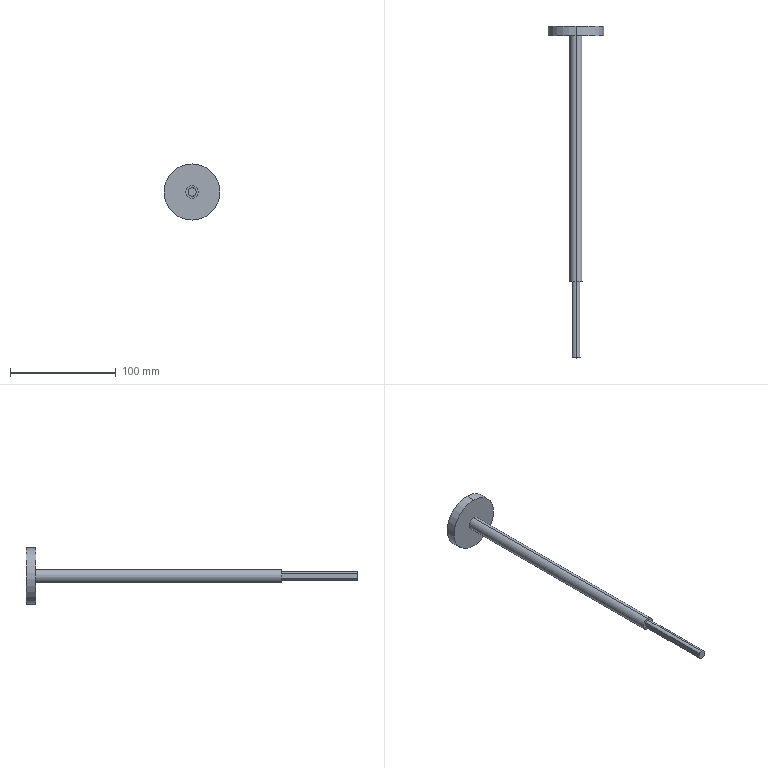Part | STEP file | 1 solid | 12 faces | box 53 x 313.9 x 53 mm | volume 49554 mm3 | cylinder 7 | plane 5 | commonest cylinder face diameters 8 x3 12 x2 53 x2
STEP:
#1=CARTESIAN_POINT('',(0.,0.,0.));
#2=DIRECTION('',(0.,0.,1.));
#3=DIRECTION('',(1.,0.,0.));
#4=AXIS2_PLACEMENT_3D('',#1,#2,#3);
#5=CARTESIAN_POINT('',(0.,313.9,-26.5));
#6=VERTEX_POINT('',#5);
#7=CARTESIAN_POINT('',(0.,313.9,26.5));
#8=VERTEX_POINT('',#7);
#9=CARTESIAN_POINT('',(0.,313.9,0.));
#10=DIRECTION('',(0.,-1.,0.));
#11=DIRECTION('',(0.,0.,-1.));
#12=AXIS2_PLACEMENT_3D('',#9,#10,#11);
#13=CIRCLE('',#12,26.5);
#14=CARTESIAN_POINT('',(0.,0.,0.));
#15=DIRECTION('',(0.,-1.,0.));
#16=DIRECTION('',(0.,0.,-1.));
#17=AXIS2_PLACEMENT_3D('',#14,#15,#16);
#18=CYLINDRICAL_SURFACE('',#17,26.5);
#19=CARTESIAN_POINT('',(0.,-313.9));
#20=DIRECTION('',(1.,0.));
#21=VECTOR('',#20,1.);
#22=LINE('',#19,#21);
#23=(GEOMETRIC_REPRESENTATION_CONTEXT(2)PARAMETRIC_REPRESENTATION_CONTEXT()REPRESENTATION_CONTEXT('',''));
#24=DEFINITIONAL_REPRESENTATION('',(#22),#23);
#25=PCURVE('',#18,#24);
#26=CARTESIAN_POINT('',(26.5,313.9,0.));
#27=DIRECTION('',(0.,1.,0.));
#28=DIRECTION('',(0.,0.,1.));
#29=AXIS2_PLACEMENT_3D('',#26,#27,#28);
#30=PLANE('',#29);
#31=CARTESIAN_POINT('',(-26.5,-26.5));
#32=CARTESIAN_POINT('',(-26.5,19.399));
#33=CARTESIAN_POINT('',(13.25,-3.55));
#34=CARTESIAN_POINT('',(53.,-26.5));
#35=CARTESIAN_POINT('',(13.25,-49.45));
#36=CARTESIAN_POINT('',(-26.5,-72.399));
#37=CARTESIAN_POINT('',(-26.5,-26.5));
#38=(BOUNDED_CURVE()B_SPLINE_CURVE(2,(#31,#32,#33,#34,#35,#36,#37),.UNSPECIFIED.,.T.,.F.)B_SPLINE_CURVE_WITH_KNOTS((1,2,2,2,2,1),(-2.094,0.,2.094,4.189,6.283,8.378),.UNSPECIFIED.)CURVE()GEOMETRIC_REPRESENTATION_ITEM()RATIONAL_B_SPLINE_CURVE((1.,0.5,1.,0.5,1.,0.5,1.))REPRESENTATION_ITEM(''));
#39=(GEOMETRIC_REPRESENTATION_CONTEXT(2)PARAMETRIC_REPRESENTATION_CONTEXT()REPRESENTATION_CONTEXT('',''));
#40=DEFINITIONAL_REPRESENTATION('',(#38),#39);
#41=PCURVE('',#30,#40);
#42=SURFACE_CURVE('',#13,(#25,#41),.PCURVE_S1.);
#43=EDGE_CURVE('',#6,#8,#42,.T.);
#44=ORIENTED_EDGE('',*,*,#43,.T.);
#45=CARTESIAN_POINT('',(0.,304.9,26.5));
#46=VERTEX_POINT('',#45);
#47=CARTESIAN_POINT('',(0.,0.,26.5));
#48=DIRECTION('',(0.,-1.,0.));
#49=VECTOR('',#48,1.);
#50=LINE('',#47,#49);
#51=CARTESIAN_POINT('',(3.142,0.));
#52=DIRECTION('',(0.,1.));
#53=VECTOR('',#52,1.);
#54=LINE('',#51,#53);
#55=(GEOMETRIC_REPRESENTATION_CONTEXT(2)PARAMETRIC_REPRESENTATION_CONTEXT()REPRESENTATION_CONTEXT('',''));
#56=DEFINITIONAL_REPRESENTATION('',(#54),#55);
#57=PCURVE('',#18,#56);
#58=CARTESIAN_POINT('',(0.,0.,0.));
#59=DIRECTION('',(0.,-1.,0.));
#60=DIRECTION('',(0.,0.,-1.));
#61=AXIS2_PLACEMENT_3D('',#58,#59,#60);
#62=CYLINDRICAL_SURFACE('',#61,26.5);
#63=CARTESIAN_POINT('',(3.142,0.));
#64=DIRECTION('',(0.,1.));
#65=VECTOR('',#64,1.);
#66=LINE('',#63,#65);
#67=(GEOMETRIC_REPRESENTATION_CONTEXT(2)PARAMETRIC_REPRESENTATION_CONTEXT()REPRESENTATION_CONTEXT('',''));
#68=DEFINITIONAL_REPRESENTATION('',(#66),#67);
#69=PCURVE('',#62,#68);
#70=SURFACE_CURVE('',#50,(#57,#69),.PCURVE_S1.);
#71=EDGE_CURVE('',#8,#46,#70,.T.);
#72=ORIENTED_EDGE('',*,*,#71,.T.);
#73=CARTESIAN_POINT('',(0.,304.9,-26.5));
#74=VERTEX_POINT('',#73);
#75=CARTESIAN_POINT('',(0.,304.9,0.));
#76=DIRECTION('',(0.,-1.,0.));
#77=DIRECTION('',(0.,0.,-1.));
#78=AXIS2_PLACEMENT_3D('',#75,#76,#77);
#79=CIRCLE('',#78,26.5);
#80=CARTESIAN_POINT('',(0.,-304.9));
#81=DIRECTION('',(1.,0.));
#82=VECTOR('',#81,1.);
#83=LINE('',#80,#82);
#84=(GEOMETRIC_REPRESENTATION_CONTEXT(2)PARAMETRIC_REPRESENTATION_CONTEXT()REPRESENTATION_CONTEXT('',''));
#85=DEFINITIONAL_REPRESENTATION('',(#83),#84);
#86=PCURVE('',#18,#85);
#87=CARTESIAN_POINT('',(6.,304.9,0.));
#88=DIRECTION('',(0.,-1.,0.));
#89=DIRECTION('',(0.,0.,-1.));
#90=AXIS2_PLACEMENT_3D('',#87,#88,#89);
#91=PLANE('',#90);
#92=CARTESIAN_POINT('',(0.,-6.));
#93=DIRECTION('',(1.,0.));
#94=AXIS2_PLACEMENT_2D('',#92,#93);
#95=CIRCLE('',#94,26.5);
#96=(GEOMETRIC_REPRESENTATION_CONTEXT(2)PARAMETRIC_REPRESENTATION_CONTEXT()REPRESENTATION_CONTEXT('',''));
#97=DEFINITIONAL_REPRESENTATION('',(#95),#96);
#98=PCURVE('',#91,#97);
#99=SURFACE_CURVE('',#79,(#86,#98),.PCURVE_S1.);
#100=EDGE_CURVE('',#74,#46,#99,.T.);
#101=ORIENTED_EDGE('',*,*,#100,.F.);
#102=CARTESIAN_POINT('',(0.,0.,-26.5));
#103=DIRECTION('',(0.,-1.,0.));
#104=VECTOR('',#103,1.);
#105=LINE('',#102,#104);
#106=CARTESIAN_POINT('',(0.,0.));
#107=DIRECTION('',(0.,1.));
#108=VECTOR('',#107,1.);
#109=LINE('',#106,#108);
#110=(GEOMETRIC_REPRESENTATION_CONTEXT(2)PARAMETRIC_REPRESENTATION_CONTEXT()REPRESENTATION_CONTEXT('',''));
#111=DEFINITIONAL_REPRESENTATION('',(#109),#110);
#112=PCURVE('',#18,#111);
#113=CARTESIAN_POINT('',(6.283,0.));
#114=DIRECTION('',(0.,1.));
#115=VECTOR('',#114,1.);
#116=LINE('',#113,#115);
#117=(GEOMETRIC_REPRESENTATION_CONTEXT(2)PARAMETRIC_REPRESENTATION_CONTEXT()REPRESENTATION_CONTEXT('',''));
#118=DEFINITIONAL_REPRESENTATION('',(#116),#117);
#119=PCURVE('',#62,#118);
#120=SURFACE_CURVE('',#105,(#112,#119),.PCURVE_S1.);
#121=EDGE_CURVE('',#6,#74,#120,.T.);
#122=ORIENTED_EDGE('',*,*,#121,.F.);
#123=EDGE_LOOP('',(#44,#72,#101,#122));
#124=FACE_BOUND('',#123,.T.);
#125=ADVANCED_FACE('',(#124),#18,.T.);
#126=CARTESIAN_POINT('',(0.,304.9,-6.));
#127=VERTEX_POINT('',#126);
#128=CARTESIAN_POINT('',(0.,304.9,6.));
#129=VERTEX_POINT('',#128);
#130=CARTESIAN_POINT('',(0.,304.9,0.));
#131=DIRECTION('',(0.,-1.,0.));
#132=DIRECTION('',(0.,0.,-1.));
#133=AXIS2_PLACEMENT_3D('',#130,#131,#132);
#134=CIRCLE('',#133,6.);
#135=CARTESIAN_POINT('',(0.,0.,0.));
#136=DIRECTION('',(0.,-1.,0.));
#137=DIRECTION('',(0.,0.,-1.));
#138=AXIS2_PLACEMENT_3D('',#135,#136,#137);
#139=CYLINDRICAL_SURFACE('',#138,6.);
#140=CARTESIAN_POINT('',(0.,-304.9));
#141=DIRECTION('',(1.,0.));
#142=VECTOR('',#141,1.);
#143=LINE('',#140,#142);
#144=(GEOMETRIC_REPRESENTATION_CONTEXT(2)PARAMETRIC_REPRESENTATION_CONTEXT()REPRESENTATION_CONTEXT('',''));
#145=DEFINITIONAL_REPRESENTATION('',(#143),#144);
#146=PCURVE('',#139,#145);
#147=CARTESIAN_POINT('',(0.,-6.));
#148=DIRECTION('',(1.,0.));
#149=AXIS2_PLACEMENT_2D('',#147,#148);
#150=CIRCLE('',#149,6.);
#151=(GEOMETRIC_REPRESENTATION_CONTEXT(2)PARAMETRIC_REPRESENTATION_CONTEXT()REPRESENTATION_CONTEXT('',''));
#152=DEFINITIONAL_REPRESENTATION('',(#150),#151);
#153=PCURVE('',#91,#152);
#154=SURFACE_CURVE('',#134,(#146,#153),.PCURVE_S1.);
#155=EDGE_CURVE('',#127,#129,#154,.T.);
#156=ORIENTED_EDGE('',*,*,#155,.T.);
#157=CARTESIAN_POINT('',(0.,72.,6.));
#158=VERTEX_POINT('',#157);
#159=CARTESIAN_POINT('',(0.,0.,6.));
#160=DIRECTION('',(0.,-1.,0.));
#161=VECTOR('',#160,1.);
#162=LINE('',#159,#161);
#163=CARTESIAN_POINT('',(3.142,0.));
#164=DIRECTION('',(0.,1.));
#165=VECTOR('',#164,1.);
#166=LINE('',#163,#165);
#167=(GEOMETRIC_REPRESENTATION_CONTEXT(2)PARAMETRIC_REPRESENTATION_CONTEXT()REPRESENTATION_CONTEXT('',''));
#168=DEFINITIONAL_REPRESENTATION('',(#166),#167);
#169=PCURVE('',#139,#168);
#170=CARTESIAN_POINT('',(0.,0.,0.));
#171=DIRECTION('',(0.,-1.,0.));
#172=DIRECTION('',(0.,0.,-1.));
#173=AXIS2_PLACEMENT_3D('',#170,#171,#172);
#174=CYLINDRICAL_SURFACE('',#173,6.);
#175=CARTESIAN_POINT('',(3.142,0.));
#176=DIRECTION('',(0.,1.));
#177=VECTOR('',#176,1.);
#178=LINE('',#175,#177);
#179=(GEOMETRIC_REPRESENTATION_CONTEXT(2)PARAMETRIC_REPRESENTATION_CONTEXT()REPRESENTATION_CONTEXT('',''));
#180=DEFINITIONAL_REPRESENTATION('',(#178),#179);
#181=PCURVE('',#174,#180);
#182=SURFACE_CURVE('',#162,(#169,#181),.PCURVE_S1.);
#183=EDGE_CURVE('',#129,#158,#182,.T.);
#184=ORIENTED_EDGE('',*,*,#183,.T.);
#185=CARTESIAN_POINT('',(0.,72.,-6.));
#186=VERTEX_POINT('',#185);
#187=CARTESIAN_POINT('',(0.,72.,0.));
#188=DIRECTION('',(0.,-1.,0.));
#189=DIRECTION('',(0.,0.,-1.));
#190=AXIS2_PLACEMENT_3D('',#187,#188,#189);
#191=CIRCLE('',#190,6.);
#192=CARTESIAN_POINT('',(0.,-72.));
#193=DIRECTION('',(1.,0.));
#194=VECTOR('',#193,1.);
#195=LINE('',#192,#194);
#196=(GEOMETRIC_REPRESENTATION_CONTEXT(2)PARAMETRIC_REPRESENTATION_CONTEXT()REPRESENTATION_CONTEXT('',''));
#197=DEFINITIONAL_REPRESENTATION('',(#195),#196);
#198=PCURVE('',#139,#197);
#199=CARTESIAN_POINT('',(4.,72.,0.));
#200=DIRECTION('',(0.,-1.,0.));
#201=DIRECTION('',(0.,0.,-1.));
#202=AXIS2_PLACEMENT_3D('',#199,#200,#201);
#203=PLANE('',#202);
#204=CARTESIAN_POINT('',(0.,-4.));
#205=DIRECTION('',(1.,0.));
#206=AXIS2_PLACEMENT_2D('',#204,#205);
#207=CIRCLE('',#206,6.);
#208=(GEOMETRIC_REPRESENTATION_CONTEXT(2)PARAMETRIC_REPRESENTATION_CONTEXT()REPRESENTATION_CONTEXT('',''));
#209=DEFINITIONAL_REPRESENTATION('',(#207),#208);
#210=PCURVE('',#203,#209);
#211=SURFACE_CURVE('',#191,(#198,#210),.PCURVE_S1.);
#212=EDGE_CURVE('',#186,#158,#211,.T.);
#213=ORIENTED_EDGE('',*,*,#212,.F.);
#214=CARTESIAN_POINT('',(0.,0.,-6.));
#215=DIRECTION('',(0.,-1.,0.));
#216=VECTOR('',#215,1.);
#217=LINE('',#214,#216);
#218=CARTESIAN_POINT('',(0.,0.));
#219=DIRECTION('',(0.,1.));
#220=VECTOR('',#219,1.);
#221=LINE('',#218,#220);
#222=(GEOMETRIC_REPRESENTATION_CONTEXT(2)PARAMETRIC_REPRESENTATION_CONTEXT()REPRESENTATION_CONTEXT('',''));
#223=DEFINITIONAL_REPRESENTATION('',(#221),#222);
#224=PCURVE('',#139,#223);
#225=CARTESIAN_POINT('',(6.283,0.));
#226=DIRECTION('',(0.,1.));
#227=VECTOR('',#226,1.);
#228=LINE('',#225,#227);
#229=(GEOMETRIC_REPRESENTATION_CONTEXT(2)PARAMETRIC_REPRESENTATION_CONTEXT()REPRESENTATION_CONTEXT('',''));
#230=DEFINITIONAL_REPRESENTATION('',(#228),#229);
#231=PCURVE('',#174,#230);
#232=SURFACE_CURVE('',#217,(#224,#231),.PCURVE_S1.);
#233=EDGE_CURVE('',#127,#186,#232,.T.);
#234=ORIENTED_EDGE('',*,*,#233,.F.);
#235=EDGE_LOOP('',(#156,#184,#213,#234));
#236=FACE_BOUND('',#235,.T.);
#237=ADVANCED_FACE('',(#236),#139,.T.);
#238=CARTESIAN_POINT('',(0.,72.,-4.));
#239=VERTEX_POINT('',#238);
#240=CARTESIAN_POINT('',(0.,72.,4.));
#241=VERTEX_POINT('',#240);
#242=CARTESIAN_POINT('',(0.,72.,0.));
#243=DIRECTION('',(0.,-1.,0.));
#244=DIRECTION('',(0.,0.,-1.));
#245=AXIS2_PLACEMENT_3D('',#242,#243,#244);
#246=CIRCLE('',#245,4.);
#247=CARTESIAN_POINT('',(0.,0.,0.));
#248=DIRECTION('',(0.,-1.,0.));
#249=DIRECTION('',(0.,0.,-1.));
#250=AXIS2_PLACEMENT_3D('',#247,#248,#249);
#251=CYLINDRICAL_SURFACE('',#250,4.);
#252=CARTESIAN_POINT('',(0.,-72.));
#253=DIRECTION('',(1.,0.));
#254=VECTOR('',#253,1.);
#255=LINE('',#252,#254);
#256=(GEOMETRIC_REPRESENTATION_CONTEXT(2)PARAMETRIC_REPRESENTATION_CONTEXT()REPRESENTATION_CONTEXT('',''));
#257=DEFINITIONAL_REPRESENTATION('',(#255),#256);
#258=PCURVE('',#251,#257);
#259=CARTESIAN_POINT('',(0.,-4.));
#260=DIRECTION('',(1.,0.));
#261=AXIS2_PLACEMENT_2D('',#259,#260);
#262=CIRCLE('',#261,4.);
#263=(GEOMETRIC_REPRESENTATION_CONTEXT(2)PARAMETRIC_REPRESENTATION_CONTEXT()REPRESENTATION_CONTEXT('',''));
#264=DEFINITIONAL_REPRESENTATION('',(#262),#263);
#265=PCURVE('',#203,#264);
#266=SURFACE_CURVE('',#246,(#258,#265),.PCURVE_S1.);
#267=EDGE_CURVE('',#239,#241,#266,.T.);
#268=ORIENTED_EDGE('',*,*,#267,.T.);
#269=CARTESIAN_POINT('',(0.,0.,4.));
#270=VERTEX_POINT('',#269);
#271=CARTESIAN_POINT('',(0.,0.,4.));
#272=DIRECTION('',(0.,-1.,0.));
#273=VECTOR('',#272,1.);
#274=LINE('',#271,#273);
#275=CARTESIAN_POINT('',(3.142,0.));
#276=DIRECTION('',(0.,1.));
#277=VECTOR('',#276,1.);
#278=LINE('',#275,#277);
#279=(GEOMETRIC_REPRESENTATION_CONTEXT(2)PARAMETRIC_REPRESENTATION_CONTEXT()REPRESENTATION_CONTEXT('',''));
#280=DEFINITIONAL_REPRESENTATION('',(#278),#279);
#281=PCURVE('',#251,#280);
#282=CARTESIAN_POINT('',(0.,0.,0.));
#283=DIRECTION('',(0.,-1.,0.));
#284=DIRECTION('',(0.,0.,-1.));
#285=AXIS2_PLACEMENT_3D('',#282,#283,#284);
#286=CYLINDRICAL_SURFACE('',#285,4.);
#287=CARTESIAN_POINT('',(3.142,0.));
#288=DIRECTION('',(0.,1.));
#289=VECTOR('',#288,1.);
#290=LINE('',#287,#289);
#291=(GEOMETRIC_REPRESENTATION_CONTEXT(2)PARAMETRIC_REPRESENTATION_CONTEXT()REPRESENTATION_CONTEXT('',''));
#292=DEFINITIONAL_REPRESENTATION('',(#290),#291);
#293=PCURVE('',#286,#292);
#294=SURFACE_CURVE('',#274,(#281,#293),.PCURVE_S1.);
#295=EDGE_CURVE('',#241,#270,#294,.T.);
#296=ORIENTED_EDGE('',*,*,#295,.T.);
#297=CARTESIAN_POINT('',(0.,0.,-4.));
#298=VERTEX_POINT('',#297);
#299=CARTESIAN_POINT('',(0.,0.,0.));
#300=DIRECTION('',(0.,-1.,0.));
#301=DIRECTION('',(0.,0.,-1.));
#302=AXIS2_PLACEMENT_3D('',#299,#300,#301);
#303=CIRCLE('',#302,4.);
#304=CARTESIAN_POINT('',(0.,0.));
#305=DIRECTION('',(1.,0.));
#306=VECTOR('',#305,1.);
#307=LINE('',#304,#306);
#308=(GEOMETRIC_REPRESENTATION_CONTEXT(2)PARAMETRIC_REPRESENTATION_CONTEXT()REPRESENTATION_CONTEXT('',''));
#309=DEFINITIONAL_REPRESENTATION('',(#307),#308);
#310=PCURVE('',#251,#309);
#311=CARTESIAN_POINT('',(0.,0.,0.));
#312=DIRECTION('',(0.,-1.,0.));
#313=DIRECTION('',(0.,0.,-1.));
#314=AXIS2_PLACEMENT_3D('',#311,#312,#313);
#315=PLANE('',#314);
#316=CARTESIAN_POINT('',(0.,0.));
#317=DIRECTION('',(1.,0.));
#318=AXIS2_PLACEMENT_2D('',#316,#317);
#319=CIRCLE('',#318,4.);
#320=(GEOMETRIC_REPRESENTATION_CONTEXT(2)PARAMETRIC_REPRESENTATION_CONTEXT()REPRESENTATION_CONTEXT('',''));
#321=DEFINITIONAL_REPRESENTATION('',(#319),#320);
#322=PCURVE('',#315,#321);
#323=SURFACE_CURVE('',#303,(#310,#322),.PCURVE_S1.);
#324=EDGE_CURVE('',#298,#270,#323,.T.);
#325=ORIENTED_EDGE('',*,*,#324,.F.);
#326=CARTESIAN_POINT('',(0.,0.,-4.));
#327=DIRECTION('',(0.,-1.,0.));
#328=VECTOR('',#327,1.);
#329=LINE('',#326,#328);
#330=CARTESIAN_POINT('',(0.,0.));
#331=DIRECTION('',(0.,1.));
#332=VECTOR('',#331,1.);
#333=LINE('',#330,#332);
#334=(GEOMETRIC_REPRESENTATION_CONTEXT(2)PARAMETRIC_REPRESENTATION_CONTEXT()REPRESENTATION_CONTEXT('',''));
#335=DEFINITIONAL_REPRESENTATION('',(#333),#334);
#336=PCURVE('',#251,#335);
#337=CARTESIAN_POINT('',(0.,0.,0.));
#338=DIRECTION('',(0.,-1.,0.));
#339=DIRECTION('',(0.,0.,-1.));
#340=AXIS2_PLACEMENT_3D('',#337,#338,#339);
#341=CYLINDRICAL_SURFACE('',#340,4.);
#342=CARTESIAN_POINT('',(6.283,0.));
#343=DIRECTION('',(0.,1.));
#344=VECTOR('',#343,1.);
#345=LINE('',#342,#344);
#346=(GEOMETRIC_REPRESENTATION_CONTEXT(2)PARAMETRIC_REPRESENTATION_CONTEXT()REPRESENTATION_CONTEXT('',''));
#347=DEFINITIONAL_REPRESENTATION('',(#345),#346);
#348=PCURVE('',#341,#347);
#349=SURFACE_CURVE('',#329,(#336,#348),.PCURVE_S1.);
#350=EDGE_CURVE('',#239,#298,#349,.T.);
#351=ORIENTED_EDGE('',*,*,#350,.F.);
#352=EDGE_LOOP('',(#268,#296,#325,#351));
#353=FACE_BOUND('',#352,.T.);
#354=ADVANCED_FACE('',(#353),#251,.T.);
#355=CARTESIAN_POINT('',(-3.,72.,-2.646));
#356=VERTEX_POINT('',#355);
#357=CARTESIAN_POINT('',(0.,72.,0.));
#358=DIRECTION('',(0.,-1.,0.));
#359=DIRECTION('',(0.,0.,-1.));
#360=AXIS2_PLACEMENT_3D('',#357,#358,#359);
#361=CIRCLE('',#360,4.);
#362=CARTESIAN_POINT('',(0.,-72.));
#363=DIRECTION('',(1.,0.));
#364=VECTOR('',#363,1.);
#365=LINE('',#362,#364);
#366=(GEOMETRIC_REPRESENTATION_CONTEXT(2)PARAMETRIC_REPRESENTATION_CONTEXT()REPRESENTATION_CONTEXT('',''));
#367=DEFINITIONAL_REPRESENTATION('',(#365),#366);
#368=PCURVE('',#341,#367);
#369=CARTESIAN_POINT('',(0.,-4.));
#370=DIRECTION('',(1.,0.));
#371=AXIS2_PLACEMENT_2D('',#369,#370);
#372=CIRCLE('',#371,4.);
#373=(GEOMETRIC_REPRESENTATION_CONTEXT(2)PARAMETRIC_REPRESENTATION_CONTEXT()REPRESENTATION_CONTEXT('',''));
#374=DEFINITIONAL_REPRESENTATION('',(#372),#373);
#375=PCURVE('',#203,#374);
#376=SURFACE_CURVE('',#361,(#368,#375),.PCURVE_S1.);
#377=EDGE_CURVE('',#356,#239,#376,.T.);
#378=ORIENTED_EDGE('',*,*,#377,.T.);
#379=ORIENTED_EDGE('',*,*,#350,.T.);
#380=CARTESIAN_POINT('',(-3.,0.,-2.646));
#381=VERTEX_POINT('',#380);
#382=CARTESIAN_POINT('',(0.,0.,0.));
#383=DIRECTION('',(0.,-1.,0.));
#384=DIRECTION('',(0.,0.,-1.));
#385=AXIS2_PLACEMENT_3D('',#382,#383,#384);
#386=CIRCLE('',#385,4.);
#387=CARTESIAN_POINT('',(0.,0.));
#388=DIRECTION('',(1.,0.));
#389=VECTOR('',#388,1.);
#390=LINE('',#387,#389);
#391=(GEOMETRIC_REPRESENTATION_CONTEXT(2)PARAMETRIC_REPRESENTATION_CONTEXT()REPRESENTATION_CONTEXT('',''));
#392=DEFINITIONAL_REPRESENTATION('',(#390),#391);
#393=PCURVE('',#341,#392);
#394=CARTESIAN_POINT('',(0.,0.));
#395=DIRECTION('',(1.,0.));
#396=AXIS2_PLACEMENT_2D('',#394,#395);
#397=CIRCLE('',#396,4.);
#398=(GEOMETRIC_REPRESENTATION_CONTEXT(2)PARAMETRIC_REPRESENTATION_CONTEXT()REPRESENTATION_CONTEXT('',''));
#399=DEFINITIONAL_REPRESENTATION('',(#397),#398);
#400=PCURVE('',#315,#399);
#401=SURFACE_CURVE('',#386,(#393,#400),.PCURVE_S1.);
#402=EDGE_CURVE('',#381,#298,#401,.T.);
#403=ORIENTED_EDGE('',*,*,#402,.F.);
#404=CARTESIAN_POINT('',(-3.,0.,-2.646));
#405=DIRECTION('',(0.,-1.,0.));
#406=VECTOR('',#405,1.);
#407=LINE('',#404,#406);
#408=CARTESIAN_POINT('',(5.435,0.));
#409=DIRECTION('',(0.,1.));
#410=VECTOR('',#409,1.);
#411=LINE('',#408,#410);
#412=(GEOMETRIC_REPRESENTATION_CONTEXT(2)PARAMETRIC_REPRESENTATION_CONTEXT()REPRESENTATION_CONTEXT('',''));
#413=DEFINITIONAL_REPRESENTATION('',(#411),#412);
#414=PCURVE('',#341,#413);
#415=CARTESIAN_POINT('',(-3.,95.111,11.649));
#416=DIRECTION('',(1.,0.,0.));
#417=DIRECTION('',(0.,0.,-1.));
#418=AXIS2_PLACEMENT_3D('',#415,#416,#417);
#419=PLANE('',#418);
#420=CARTESIAN_POINT('',(14.294,-95.111));
#421=DIRECTION('',(0.,-1.));
#422=VECTOR('',#421,1.);
#423=LINE('',#420,#422);
#424=(GEOMETRIC_REPRESENTATION_CONTEXT(2)PARAMETRIC_REPRESENTATION_CONTEXT()REPRESENTATION_CONTEXT('',''));
#425=DEFINITIONAL_REPRESENTATION('',(#423),#424);
#426=PCURVE('',#419,#425);
#427=SURFACE_CURVE('',#407,(#414,#426),.PCURVE_S1.);
#428=EDGE_CURVE('',#356,#381,#427,.T.);
#429=ORIENTED_EDGE('',*,*,#428,.F.);
#430=EDGE_LOOP('',(#378,#379,#403,#429));
#431=FACE_BOUND('',#430,.T.);
#432=ADVANCED_FACE('',(#431),#341,.T.);
#433=CARTESIAN_POINT('',(-3.,0.,2.646));
#434=VERTEX_POINT('',#433);
#435=CARTESIAN_POINT('',(-3.,0.,11.649));
#436=DIRECTION('',(0.,0.,1.));
#437=VECTOR('',#436,1.);
#438=LINE('',#435,#437);
#439=CARTESIAN_POINT('',(-11.649,-3.));
#440=DIRECTION('',(-1.,0.));
#441=VECTOR('',#440,1.);
#442=LINE('',#439,#441);
#443=(GEOMETRIC_REPRESENTATION_CONTEXT(2)PARAMETRIC_REPRESENTATION_CONTEXT()REPRESENTATION_CONTEXT('',''));
#444=DEFINITIONAL_REPRESENTATION('',(#442),#443);
#445=PCURVE('',#315,#444);
#446=CARTESIAN_POINT('',(0.,-95.111));
#447=DIRECTION('',(-1.,0.));
#448=VECTOR('',#447,1.);
#449=LINE('',#446,#448);
#450=(GEOMETRIC_REPRESENTATION_CONTEXT(2)PARAMETRIC_REPRESENTATION_CONTEXT()REPRESENTATION_CONTEXT('',''));
#451=DEFINITIONAL_REPRESENTATION('',(#449),#450);
#452=PCURVE('',#419,#451);
#453=SURFACE_CURVE('',#438,(#445,#452),.PCURVE_S1.);
#454=EDGE_CURVE('',#381,#434,#453,.T.);
#455=ORIENTED_EDGE('',*,*,#454,.F.);
#456=ORIENTED_EDGE('',*,*,#402,.T.);
#457=ORIENTED_EDGE('',*,*,#324,.T.);
#458=CARTESIAN_POINT('',(0.,0.,0.));
#459=DIRECTION('',(0.,-1.,0.));
#460=DIRECTION('',(0.,0.,-1.));
#461=AXIS2_PLACEMENT_3D('',#458,#459,#460);
#462=CIRCLE('',#461,4.);
#463=CARTESIAN_POINT('',(0.,0.));
#464=DIRECTION('',(1.,0.));
#465=AXIS2_PLACEMENT_2D('',#463,#464);
#466=CIRCLE('',#465,4.);
#467=(GEOMETRIC_REPRESENTATION_CONTEXT(2)PARAMETRIC_REPRESENTATION_CONTEXT()REPRESENTATION_CONTEXT('',''));
#468=DEFINITIONAL_REPRESENTATION('',(#466),#467);
#469=PCURVE('',#315,#468);
#470=CARTESIAN_POINT('',(0.,0.));
#471=DIRECTION('',(1.,0.));
#472=VECTOR('',#471,1.);
#473=LINE('',#470,#472);
#474=(GEOMETRIC_REPRESENTATION_CONTEXT(2)PARAMETRIC_REPRESENTATION_CONTEXT()REPRESENTATION_CONTEXT('',''));
#475=DEFINITIONAL_REPRESENTATION('',(#473),#474);
#476=PCURVE('',#286,#475);
#477=SURFACE_CURVE('',#462,(#469,#476),.PCURVE_S1.);
#478=EDGE_CURVE('',#270,#434,#477,.T.);
#479=ORIENTED_EDGE('',*,*,#478,.T.);
#480=EDGE_LOOP('',(#455,#456,#457,#479));
#481=FACE_BOUND('',#480,.T.);
#482=ADVANCED_FACE('',(#481),#315,.T.);
#483=ORIENTED_EDGE('',*,*,#295,.F.);
#484=CARTESIAN_POINT('',(-3.,72.,2.646));
#485=VERTEX_POINT('',#484);
#486=CARTESIAN_POINT('',(0.,72.,0.));
#487=DIRECTION('',(0.,-1.,0.));
#488=DIRECTION('',(0.,0.,-1.));
#489=AXIS2_PLACEMENT_3D('',#486,#487,#488);
#490=CIRCLE('',#489,4.);
#491=CARTESIAN_POINT('',(0.,-72.));
#492=DIRECTION('',(1.,0.));
#493=VECTOR('',#492,1.);
#494=LINE('',#491,#493);
#495=(GEOMETRIC_REPRESENTATION_CONTEXT(2)PARAMETRIC_REPRESENTATION_CONTEXT()REPRESENTATION_CONTEXT('',''));
#496=DEFINITIONAL_REPRESENTATION('',(#494),#495);
#497=PCURVE('',#286,#496);
#498=CARTESIAN_POINT('',(0.,-4.));
#499=DIRECTION('',(1.,0.));
#500=AXIS2_PLACEMENT_2D('',#498,#499);
#501=CIRCLE('',#500,4.);
#502=(GEOMETRIC_REPRESENTATION_CONTEXT(2)PARAMETRIC_REPRESENTATION_CONTEXT()REPRESENTATION_CONTEXT('',''));
#503=DEFINITIONAL_REPRESENTATION('',(#501),#502);
#504=PCURVE('',#203,#503);
#505=SURFACE_CURVE('',#490,(#497,#504),.PCURVE_S1.);
#506=EDGE_CURVE('',#241,#485,#505,.T.);
#507=ORIENTED_EDGE('',*,*,#506,.T.);
#508=CARTESIAN_POINT('',(-3.,0.,2.646));
#509=DIRECTION('',(0.,1.,0.));
#510=VECTOR('',#509,1.);
#511=LINE('',#508,#510);
#512=CARTESIAN_POINT('',(3.99,0.));
#513=DIRECTION('',(0.,-1.));
#514=VECTOR('',#513,1.);
#515=LINE('',#512,#514);
#516=(GEOMETRIC_REPRESENTATION_CONTEXT(2)PARAMETRIC_REPRESENTATION_CONTEXT()REPRESENTATION_CONTEXT('',''));
#517=DEFINITIONAL_REPRESENTATION('',(#515),#516);
#518=PCURVE('',#286,#517);
#519=CARTESIAN_POINT('',(9.003,-95.111));
#520=DIRECTION('',(0.,1.));
#521=VECTOR('',#520,1.);
#522=LINE('',#519,#521);
#523=(GEOMETRIC_REPRESENTATION_CONTEXT(2)PARAMETRIC_REPRESENTATION_CONTEXT()REPRESENTATION_CONTEXT('',''));
#524=DEFINITIONAL_REPRESENTATION('',(#522),#523);
#525=PCURVE('',#419,#524);
#526=SURFACE_CURVE('',#511,(#518,#525),.PCURVE_S1.);
#527=EDGE_CURVE('',#434,#485,#526,.T.);
#528=ORIENTED_EDGE('',*,*,#527,.F.);
#529=ORIENTED_EDGE('',*,*,#478,.F.);
#530=EDGE_LOOP('',(#483,#507,#528,#529));
#531=FACE_BOUND('',#530,.T.);
#532=ADVANCED_FACE('',(#531),#286,.T.);
#533=ORIENTED_EDGE('',*,*,#377,.F.);
#534=CARTESIAN_POINT('',(-3.,72.,11.649));
#535=DIRECTION('',(0.,0.,-1.));
#536=VECTOR('',#535,1.);
#537=LINE('',#534,#536);
#538=CARTESIAN_POINT('',(-11.649,-7.));
#539=DIRECTION('',(1.,0.));
#540=VECTOR('',#539,1.);
#541=LINE('',#538,#540);
#542=(GEOMETRIC_REPRESENTATION_CONTEXT(2)PARAMETRIC_REPRESENTATION_CONTEXT()REPRESENTATION_CONTEXT('',''));
#543=DEFINITIONAL_REPRESENTATION('',(#541),#542);
#544=PCURVE('',#203,#543);
#545=CARTESIAN_POINT('',(0.,-23.111));
#546=DIRECTION('',(1.,0.));
#547=VECTOR('',#546,1.);
#548=LINE('',#545,#547);
#549=(GEOMETRIC_REPRESENTATION_CONTEXT(2)PARAMETRIC_REPRESENTATION_CONTEXT()REPRESENTATION_CONTEXT('',''));
#550=DEFINITIONAL_REPRESENTATION('',(#548),#549);
#551=PCURVE('',#419,#550);
#552=SURFACE_CURVE('',#537,(#544,#551),.PCURVE_S1.);
#553=EDGE_CURVE('',#485,#356,#552,.T.);
#554=ORIENTED_EDGE('',*,*,#553,.F.);
#555=ORIENTED_EDGE('',*,*,#506,.F.);
#556=ORIENTED_EDGE('',*,*,#267,.F.);
#557=EDGE_LOOP('',(#533,#554,#555,#556));
#558=FACE_BOUND('',#557,.T.);
#559=ORIENTED_EDGE('',*,*,#212,.T.);
#560=CARTESIAN_POINT('',(0.,72.,0.));
#561=DIRECTION('',(0.,-1.,0.));
#562=DIRECTION('',(0.,0.,-1.));
#563=AXIS2_PLACEMENT_3D('',#560,#561,#562);
#564=CIRCLE('',#563,6.);
#565=CARTESIAN_POINT('',(0.,-4.));
#566=DIRECTION('',(1.,0.));
#567=AXIS2_PLACEMENT_2D('',#565,#566);
#568=CIRCLE('',#567,6.);
#569=(GEOMETRIC_REPRESENTATION_CONTEXT(2)PARAMETRIC_REPRESENTATION_CONTEXT()REPRESENTATION_CONTEXT('',''));
#570=DEFINITIONAL_REPRESENTATION('',(#568),#569);
#571=PCURVE('',#203,#570);
#572=CARTESIAN_POINT('',(0.,-72.));
#573=DIRECTION('',(1.,0.));
#574=VECTOR('',#573,1.);
#575=LINE('',#572,#574);
#576=(GEOMETRIC_REPRESENTATION_CONTEXT(2)PARAMETRIC_REPRESENTATION_CONTEXT()REPRESENTATION_CONTEXT('',''));
#577=DEFINITIONAL_REPRESENTATION('',(#575),#576);
#578=PCURVE('',#174,#577);
#579=SURFACE_CURVE('',#564,(#571,#578),.PCURVE_S1.);
#580=EDGE_CURVE('',#158,#186,#579,.T.);
#581=ORIENTED_EDGE('',*,*,#580,.T.);
#582=EDGE_LOOP('',(#559,#581));
#583=FACE_BOUND('',#582,.T.);
#584=ADVANCED_FACE('',(#558,#583),#203,.T.);
#585=ORIENTED_EDGE('',*,*,#183,.F.);
#586=CARTESIAN_POINT('',(0.,304.9,0.));
#587=DIRECTION('',(0.,-1.,0.));
#588=DIRECTION('',(0.,0.,-1.));
#589=AXIS2_PLACEMENT_3D('',#586,#587,#588);
#590=CIRCLE('',#589,6.);
#591=CARTESIAN_POINT('',(0.,-304.9));
#592=DIRECTION('',(1.,0.));
#593=VECTOR('',#592,1.);
#594=LINE('',#591,#593);
#595=(GEOMETRIC_REPRESENTATION_CONTEXT(2)PARAMETRIC_REPRESENTATION_CONTEXT()REPRESENTATION_CONTEXT('',''));
#596=DEFINITIONAL_REPRESENTATION('',(#594),#595);
#597=PCURVE('',#174,#596);
#598=CARTESIAN_POINT('',(0.,-6.));
#599=DIRECTION('',(1.,0.));
#600=AXIS2_PLACEMENT_2D('',#598,#599);
#601=CIRCLE('',#600,6.);
#602=(GEOMETRIC_REPRESENTATION_CONTEXT(2)PARAMETRIC_REPRESENTATION_CONTEXT()REPRESENTATION_CONTEXT('',''));
#603=DEFINITIONAL_REPRESENTATION('',(#601),#602);
#604=PCURVE('',#91,#603);
#605=SURFACE_CURVE('',#590,(#597,#604),.PCURVE_S1.);
#606=EDGE_CURVE('',#129,#127,#605,.T.);
#607=ORIENTED_EDGE('',*,*,#606,.T.);
#608=ORIENTED_EDGE('',*,*,#233,.T.);
#609=ORIENTED_EDGE('',*,*,#580,.F.);
#610=EDGE_LOOP('',(#585,#607,#608,#609));
#611=FACE_BOUND('',#610,.T.);
#612=ADVANCED_FACE('',(#611),#174,.T.);
#613=ORIENTED_EDGE('',*,*,#100,.T.);
#614=CARTESIAN_POINT('',(0.,304.9,0.));
#615=DIRECTION('',(0.,-1.,0.));
#616=DIRECTION('',(0.,0.,-1.));
#617=AXIS2_PLACEMENT_3D('',#614,#615,#616);
#618=CIRCLE('',#617,26.5);
#619=CARTESIAN_POINT('',(0.,-6.));
#620=DIRECTION('',(1.,0.));
#621=AXIS2_PLACEMENT_2D('',#619,#620);
#622=CIRCLE('',#621,26.5);
#623=(GEOMETRIC_REPRESENTATION_CONTEXT(2)PARAMETRIC_REPRESENTATION_CONTEXT()REPRESENTATION_CONTEXT('',''));
#624=DEFINITIONAL_REPRESENTATION('',(#622),#623);
#625=PCURVE('',#91,#624);
#626=CARTESIAN_POINT('',(0.,-304.9));
#627=DIRECTION('',(1.,0.));
#628=VECTOR('',#627,1.);
#629=LINE('',#626,#628);
#630=(GEOMETRIC_REPRESENTATION_CONTEXT(2)PARAMETRIC_REPRESENTATION_CONTEXT()REPRESENTATION_CONTEXT('',''));
#631=DEFINITIONAL_REPRESENTATION('',(#629),#630);
#632=PCURVE('',#62,#631);
#633=SURFACE_CURVE('',#618,(#625,#632),.PCURVE_S1.);
#634=EDGE_CURVE('',#46,#74,#633,.T.);
#635=ORIENTED_EDGE('',*,*,#634,.T.);
#636=EDGE_LOOP('',(#613,#635));
#637=FACE_BOUND('',#636,.T.);
#638=ORIENTED_EDGE('',*,*,#155,.F.);
#639=ORIENTED_EDGE('',*,*,#606,.F.);
#640=EDGE_LOOP('',(#638,#639));
#641=FACE_BOUND('',#640,.T.);
#642=ADVANCED_FACE('',(#637,#641),#91,.T.);
#643=ORIENTED_EDGE('',*,*,#71,.F.);
#644=CARTESIAN_POINT('',(0.,313.9,0.));
#645=DIRECTION('',(0.,-1.,0.));
#646=DIRECTION('',(0.,0.,-1.));
#647=AXIS2_PLACEMENT_3D('',#644,#645,#646);
#648=CIRCLE('',#647,26.5);
#649=CARTESIAN_POINT('',(0.,-313.9));
#650=DIRECTION('',(1.,0.));
#651=VECTOR('',#650,1.);
#652=LINE('',#649,#651);
#653=(GEOMETRIC_REPRESENTATION_CONTEXT(2)PARAMETRIC_REPRESENTATION_CONTEXT()REPRESENTATION_CONTEXT('',''));
#654=DEFINITIONAL_REPRESENTATION('',(#652),#653);
#655=PCURVE('',#62,#654);
#656=CARTESIAN_POINT('',(-26.5,-26.5));
#657=CARTESIAN_POINT('',(-26.5,19.399));
#658=CARTESIAN_POINT('',(13.25,-3.55));
#659=CARTESIAN_POINT('',(53.,-26.5));
#660=CARTESIAN_POINT('',(13.25,-49.45));
#661=CARTESIAN_POINT('',(-26.5,-72.399));
#662=CARTESIAN_POINT('',(-26.5,-26.5));
#663=(BOUNDED_CURVE()B_SPLINE_CURVE(2,(#656,#657,#658,#659,#660,#661,#662),.UNSPECIFIED.,.T.,.F.)B_SPLINE_CURVE_WITH_KNOTS((1,2,2,2,2,1),(-2.094,0.,2.094,4.189,6.283,8.378),.UNSPECIFIED.)CURVE()GEOMETRIC_REPRESENTATION_ITEM()RATIONAL_B_SPLINE_CURVE((1.,0.5,1.,0.5,1.,0.5,1.))REPRESENTATION_ITEM(''));
#664=(GEOMETRIC_REPRESENTATION_CONTEXT(2)PARAMETRIC_REPRESENTATION_CONTEXT()REPRESENTATION_CONTEXT('',''));
#665=DEFINITIONAL_REPRESENTATION('',(#663),#664);
#666=PCURVE('',#30,#665);
#667=SURFACE_CURVE('',#648,(#655,#666),.PCURVE_S1.);
#668=EDGE_CURVE('',#8,#6,#667,.T.);
#669=ORIENTED_EDGE('',*,*,#668,.T.);
#670=ORIENTED_EDGE('',*,*,#121,.T.);
#671=ORIENTED_EDGE('',*,*,#634,.F.);
#672=EDGE_LOOP('',(#643,#669,#670,#671));
#673=FACE_BOUND('',#672,.T.);
#674=ADVANCED_FACE('',(#673),#62,.T.);
#675=ORIENTED_EDGE('',*,*,#43,.F.);
#676=ORIENTED_EDGE('',*,*,#668,.F.);
#677=EDGE_LOOP('',(#675,#676));
#678=FACE_BOUND('',#677,.T.);
#679=ADVANCED_FACE('',(#678),#30,.T.);
#680=ORIENTED_EDGE('',*,*,#527,.T.);
#681=ORIENTED_EDGE('',*,*,#553,.T.);
#682=ORIENTED_EDGE('',*,*,#428,.T.);
#683=ORIENTED_EDGE('',*,*,#454,.T.);
#684=EDGE_LOOP('',(#680,#681,#682,#683));
#685=FACE_BOUND('',#684,.T.);
#686=ADVANCED_FACE('',(#685),#419,.F.);
#687=CLOSED_SHELL('',(#125,#237,#354,#432,#482,#532,#584,#612,#642,#674,#679,#686));
#688=MANIFOLD_SOLID_BREP('',#687);
#689=(LENGTH_UNIT()NAMED_UNIT(*)SI_UNIT(.MILLI.,.METRE.));
#690=UNCERTAINTY_MEASURE_WITH_UNIT(LENGTH_MEASURE(0.0000001),#689,'','');
#691=(NAMED_UNIT(*)PLANE_ANGLE_UNIT()SI_UNIT($,.RADIAN.));
#692=(NAMED_UNIT(*)SI_UNIT($,.STERADIAN.)SOLID_ANGLE_UNIT());
#693=(GEOMETRIC_REPRESENTATION_CONTEXT(3)GLOBAL_UNCERTAINTY_ASSIGNED_CONTEXT((#690))GLOBAL_UNIT_ASSIGNED_CONTEXT((#689,#691,#692))REPRESENTATION_CONTEXT('',''));
#694=ADVANCED_BREP_SHAPE_REPRESENTATION('',(#4,#688),#693);